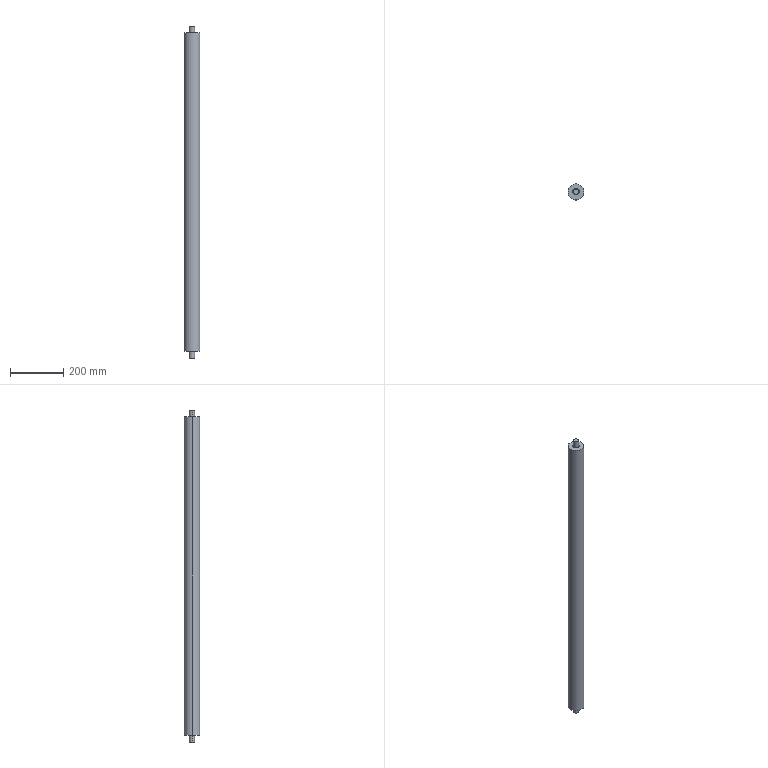Part | SolidWorks | features ICE 2, Extrusion 1, MirrorPattern 1 | 2 solids | 16 faces | box 60 x 60 x 1250 mm | volume 3405863 mm3 | cylinder 10 | plane 6 | commonest cylinder face diameters 20 x4 24 x4 60 x2
STEP:
#1=CARTESIAN_POINT('',(10.,0.,625.));
#2=VERTEX_POINT('',#1);
#3=CARTESIAN_POINT('',(-10.,0.,625.));
#4=VERTEX_POINT('',#3);
#5=CARTESIAN_POINT('',(0.,0.,625.));
#6=DIRECTION('',(0.,0.,1.));
#7=DIRECTION('',(1.,0.,0.));
#8=AXIS2_PLACEMENT_3D('',#5,#6,#7);
#9=CIRCLE('',#8,10.);
#10=EDGE_CURVE('',#2,#4,#9,.T.);
#11=ORIENTED_EDGE('',*,*,#10,.F.);
#12=CARTESIAN_POINT('',(10.,0.,-625.));
#13=VERTEX_POINT('',#12);
#14=CARTESIAN_POINT('',(10.,0.,625.));
#15=DIRECTION('',(0.,0.,-1.));
#16=VECTOR('',#15,1000.);
#17=LINE('',#14,#16);
#18=EDGE_CURVE('',#2,#13,#17,.T.);
#19=ORIENTED_EDGE('',*,*,#18,.T.);
#20=CARTESIAN_POINT('',(-10.,0.,-625.));
#21=VERTEX_POINT('',#20);
#22=CARTESIAN_POINT('',(0.,0.,-625.));
#23=DIRECTION('',(0.,0.,1.));
#24=DIRECTION('',(1.,0.,0.));
#25=AXIS2_PLACEMENT_3D('',#22,#23,#24);
#26=CIRCLE('',#25,10.);
#27=EDGE_CURVE('',#13,#21,#26,.T.);
#28=ORIENTED_EDGE('',*,*,#27,.T.);
#29=CARTESIAN_POINT('',(-10.,0.,625.));
#30=DIRECTION('',(0.,0.,-1.));
#31=VECTOR('',#30,1000.);
#32=LINE('',#29,#31);
#33=EDGE_CURVE('',#4,#21,#32,.T.);
#34=ORIENTED_EDGE('',*,*,#33,.F.);
#35=EDGE_LOOP('',(#11,#19,#28,#34));
#36=FACE_OUTER_BOUND('',#35,.T.);
#37=CARTESIAN_POINT('',(0.,0.,625.));
#38=DIRECTION('',(0.,0.,-1.));
#39=DIRECTION('',(-1.,0.,0.));
#40=AXIS2_PLACEMENT_3D('',#37,#38,#39);
#41=CYLINDRICAL_SURFACE('',#40,10.);
#42=ADVANCED_FACE('',(#36),#41,.T.);
#43=ORIENTED_EDGE('',*,*,#18,.F.);
#44=CARTESIAN_POINT('',(0.,0.,625.));
#45=DIRECTION('',(0.,0.,1.));
#46=DIRECTION('',(1.,0.,0.));
#47=AXIS2_PLACEMENT_3D('',#44,#45,#46);
#48=CIRCLE('',#47,10.);
#49=EDGE_CURVE('',#4,#2,#48,.T.);
#50=ORIENTED_EDGE('',*,*,#49,.F.);
#51=ORIENTED_EDGE('',*,*,#33,.T.);
#52=CARTESIAN_POINT('',(0.,0.,-625.));
#53=DIRECTION('',(0.,0.,1.));
#54=DIRECTION('',(1.,0.,0.));
#55=AXIS2_PLACEMENT_3D('',#52,#53,#54);
#56=CIRCLE('',#55,10.);
#57=EDGE_CURVE('',#21,#13,#56,.T.);
#58=ORIENTED_EDGE('',*,*,#57,.T.);
#59=EDGE_LOOP('',(#43,#50,#51,#58));
#60=FACE_OUTER_BOUND('',#59,.T.);
#61=CARTESIAN_POINT('',(0.,0.,625.));
#62=DIRECTION('',(0.,0.,-1.));
#63=DIRECTION('',(-1.,0.,0.));
#64=AXIS2_PLACEMENT_3D('',#61,#62,#63);
#65=CYLINDRICAL_SURFACE('',#64,10.);
#66=ADVANCED_FACE('',(#60),#65,.T.);
#67=ORIENTED_EDGE('',*,*,#49,.T.);
#68=ORIENTED_EDGE('',*,*,#10,.T.);
#69=EDGE_LOOP('',(#67,#68));
#70=FACE_OUTER_BOUND('',#69,.T.);
#71=CARTESIAN_POINT('',(0.,0.,625.));
#72=DIRECTION('',(0.,0.,1.));
#73=DIRECTION('',(1.,0.,0.));
#74=AXIS2_PLACEMENT_3D('',#71,#72,#73);
#75=PLANE('',#74);
#76=ADVANCED_FACE('',(#70),#75,.T.);
#77=ORIENTED_EDGE('',*,*,#57,.F.);
#78=ORIENTED_EDGE('',*,*,#27,.F.);
#79=EDGE_LOOP('',(#77,#78));
#80=FACE_OUTER_BOUND('',#79,.T.);
#81=CARTESIAN_POINT('',(0.,0.,-625.));
#82=DIRECTION('',(0.,0.,1.));
#83=DIRECTION('',(1.,0.,0.));
#84=AXIS2_PLACEMENT_3D('',#81,#82,#83);
#85=PLANE('',#84);
#86=ADVANCED_FACE('',(#80),#85,.F.);
#87=CLOSED_SHELL('',(#42,#66,#76,#86));
#88=MANIFOLD_SOLID_BREP('',#87);
#89=CARTESIAN_POINT('',(-12.,0.,-590.));
#90=VERTEX_POINT('',#89);
#91=CARTESIAN_POINT('',(12.,0.,-590.));
#92=VERTEX_POINT('',#91);
#93=CARTESIAN_POINT('',(0.,0.,-590.));
#94=DIRECTION('',(0.,0.,1.));
#95=DIRECTION('',(1.,0.,0.));
#96=AXIS2_PLACEMENT_3D('',#93,#94,#95);
#97=CIRCLE('',#96,12.);
#98=EDGE_CURVE('',#90,#92,#97,.T.);
#99=ORIENTED_EDGE('',*,*,#98,.T.);
#100=CARTESIAN_POINT('',(12.,0.,-600.));
#101=VERTEX_POINT('',#100);
#102=CARTESIAN_POINT('',(12.,0.,-590.));
#103=DIRECTION('',(0.,0.,-1.));
#104=VECTOR('',#103,1000.);
#105=LINE('',#102,#104);
#106=EDGE_CURVE('',#92,#101,#105,.T.);
#107=ORIENTED_EDGE('',*,*,#106,.T.);
#108=CARTESIAN_POINT('',(-12.,0.,-600.));
#109=VERTEX_POINT('',#108);
#110=CARTESIAN_POINT('',(0.,0.,-600.));
#111=DIRECTION('',(0.,0.,1.));
#112=DIRECTION('',(1.,0.,0.));
#113=AXIS2_PLACEMENT_3D('',#110,#111,#112);
#114=CIRCLE('',#113,12.);
#115=EDGE_CURVE('',#109,#101,#114,.T.);
#116=ORIENTED_EDGE('',*,*,#115,.F.);
#117=CARTESIAN_POINT('',(-12.,0.,-590.));
#118=DIRECTION('',(0.,0.,-1.));
#119=VECTOR('',#118,1000.);
#120=LINE('',#117,#119);
#121=EDGE_CURVE('',#90,#109,#120,.T.);
#122=ORIENTED_EDGE('',*,*,#121,.F.);
#123=EDGE_LOOP('',(#99,#107,#116,#122));
#124=FACE_OUTER_BOUND('',#123,.T.);
#125=CARTESIAN_POINT('',(0.,0.,-590.));
#126=DIRECTION('',(0.,0.,-1.));
#127=DIRECTION('',(-1.,0.,0.));
#128=AXIS2_PLACEMENT_3D('',#125,#126,#127);
#129=CYLINDRICAL_SURFACE('',#128,12.);
#130=ADVANCED_FACE('',(#124),#129,.F.);
#131=CARTESIAN_POINT('',(-12.,0.,590.));
#132=VERTEX_POINT('',#131);
#133=CARTESIAN_POINT('',(12.,0.,590.));
#134=VERTEX_POINT('',#133);
#135=CARTESIAN_POINT('',(0.,0.,590.));
#136=DIRECTION('',(0.,0.,1.));
#137=DIRECTION('',(1.,0.,0.));
#138=AXIS2_PLACEMENT_3D('',#135,#136,#137);
#139=CIRCLE('',#138,12.);
#140=EDGE_CURVE('',#132,#134,#139,.T.);
#141=ORIENTED_EDGE('',*,*,#140,.F.);
#142=CARTESIAN_POINT('',(-12.,0.,600.));
#143=VERTEX_POINT('',#142);
#144=CARTESIAN_POINT('',(-12.,0.,590.));
#145=DIRECTION('',(0.,0.,1.));
#146=VECTOR('',#145,1000.);
#147=LINE('',#144,#146);
#148=EDGE_CURVE('',#132,#143,#147,.T.);
#149=ORIENTED_EDGE('',*,*,#148,.T.);
#150=CARTESIAN_POINT('',(12.,0.,600.));
#151=VERTEX_POINT('',#150);
#152=CARTESIAN_POINT('',(0.,0.,600.));
#153=DIRECTION('',(0.,0.,1.));
#154=DIRECTION('',(1.,0.,0.));
#155=AXIS2_PLACEMENT_3D('',#152,#153,#154);
#156=CIRCLE('',#155,12.);
#157=EDGE_CURVE('',#143,#151,#156,.T.);
#158=ORIENTED_EDGE('',*,*,#157,.T.);
#159=CARTESIAN_POINT('',(12.,0.,590.));
#160=DIRECTION('',(0.,0.,1.));
#161=VECTOR('',#160,1000.);
#162=LINE('',#159,#161);
#163=EDGE_CURVE('',#134,#151,#162,.T.);
#164=ORIENTED_EDGE('',*,*,#163,.F.);
#165=EDGE_LOOP('',(#141,#149,#158,#164));
#166=FACE_OUTER_BOUND('',#165,.T.);
#167=CARTESIAN_POINT('',(0.,0.,590.));
#168=DIRECTION('',(0.,0.,1.));
#169=DIRECTION('',(1.,0.,0.));
#170=AXIS2_PLACEMENT_3D('',#167,#168,#169);
#171=CYLINDRICAL_SURFACE('',#170,12.);
#172=ADVANCED_FACE('',(#166),#171,.F.);
#173=CARTESIAN_POINT('',(30.,0.,600.));
#174=VERTEX_POINT('',#173);
#175=CARTESIAN_POINT('',(-30.,0.,600.));
#176=VERTEX_POINT('',#175);
#177=CARTESIAN_POINT('',(0.,0.,600.));
#178=DIRECTION('',(0.,0.,1.));
#179=DIRECTION('',(1.,0.,0.));
#180=AXIS2_PLACEMENT_3D('',#177,#178,#179);
#181=CIRCLE('',#180,30.);
#182=EDGE_CURVE('',#174,#176,#181,.T.);
#183=ORIENTED_EDGE('',*,*,#182,.F.);
#184=CARTESIAN_POINT('',(30.,0.,-600.));
#185=VERTEX_POINT('',#184);
#186=CARTESIAN_POINT('',(30.,0.,600.));
#187=DIRECTION('',(0.,0.,-1.));
#188=VECTOR('',#187,1000.);
#189=LINE('',#186,#188);
#190=EDGE_CURVE('',#174,#185,#189,.T.);
#191=ORIENTED_EDGE('',*,*,#190,.T.);
#192=CARTESIAN_POINT('',(-30.,0.,-600.));
#193=VERTEX_POINT('',#192);
#194=CARTESIAN_POINT('',(0.,0.,-600.));
#195=DIRECTION('',(0.,0.,1.));
#196=DIRECTION('',(1.,0.,0.));
#197=AXIS2_PLACEMENT_3D('',#194,#195,#196);
#198=CIRCLE('',#197,30.);
#199=EDGE_CURVE('',#185,#193,#198,.T.);
#200=ORIENTED_EDGE('',*,*,#199,.T.);
#201=CARTESIAN_POINT('',(-30.,0.,600.));
#202=DIRECTION('',(0.,0.,-1.));
#203=VECTOR('',#202,1000.);
#204=LINE('',#201,#203);
#205=EDGE_CURVE('',#176,#193,#204,.T.);
#206=ORIENTED_EDGE('',*,*,#205,.F.);
#207=EDGE_LOOP('',(#183,#191,#200,#206));
#208=FACE_OUTER_BOUND('',#207,.T.);
#209=CARTESIAN_POINT('',(0.,0.,600.));
#210=DIRECTION('',(0.,0.,-1.));
#211=DIRECTION('',(-1.,0.,0.));
#212=AXIS2_PLACEMENT_3D('',#209,#210,#211);
#213=CYLINDRICAL_SURFACE('',#212,30.);
#214=ADVANCED_FACE('',(#208),#213,.T.);
#215=CARTESIAN_POINT('',(-10.,0.,590.));
#216=VERTEX_POINT('',#215);
#217=CARTESIAN_POINT('',(10.,0.,590.));
#218=VERTEX_POINT('',#217);
#219=CARTESIAN_POINT('',(0.,0.,590.));
#220=DIRECTION('',(0.,0.,1.));
#221=DIRECTION('',(1.,0.,0.));
#222=AXIS2_PLACEMENT_3D('',#219,#220,#221);
#223=CIRCLE('',#222,10.);
#224=EDGE_CURVE('',#216,#218,#223,.T.);
#225=ORIENTED_EDGE('',*,*,#224,.T.);
#226=CARTESIAN_POINT('',(10.,0.,-590.));
#227=VERTEX_POINT('',#226);
#228=CARTESIAN_POINT('',(10.,0.,600.));
#229=DIRECTION('',(0.,0.,-1.));
#230=VECTOR('',#229,1000.);
#231=LINE('',#228,#230);
#232=EDGE_CURVE('',#218,#227,#231,.T.);
#233=ORIENTED_EDGE('',*,*,#232,.T.);
#234=CARTESIAN_POINT('',(-10.,0.,-590.));
#235=VERTEX_POINT('',#234);
#236=CARTESIAN_POINT('',(0.,0.,-590.));
#237=DIRECTION('',(0.,0.,-1.));
#238=DIRECTION('',(-1.,0.,0.));
#239=AXIS2_PLACEMENT_3D('',#236,#237,#238);
#240=CIRCLE('',#239,10.);
#241=EDGE_CURVE('',#227,#235,#240,.T.);
#242=ORIENTED_EDGE('',*,*,#241,.T.);
#243=CARTESIAN_POINT('',(-10.,0.,600.));
#244=DIRECTION('',(0.,0.,-1.));
#245=VECTOR('',#244,1000.);
#246=LINE('',#243,#245);
#247=EDGE_CURVE('',#216,#235,#246,.T.);
#248=ORIENTED_EDGE('',*,*,#247,.F.);
#249=EDGE_LOOP('',(#225,#233,#242,#248));
#250=FACE_OUTER_BOUND('',#249,.T.);
#251=CARTESIAN_POINT('',(0.,0.,600.));
#252=DIRECTION('',(0.,0.,-1.));
#253=DIRECTION('',(-1.,0.,0.));
#254=AXIS2_PLACEMENT_3D('',#251,#252,#253);
#255=CYLINDRICAL_SURFACE('',#254,10.);
#256=ADVANCED_FACE('',(#250),#255,.F.);
#257=ORIENTED_EDGE('',*,*,#232,.F.);
#258=CARTESIAN_POINT('',(0.,0.,590.));
#259=DIRECTION('',(0.,0.,1.));
#260=DIRECTION('',(1.,0.,0.));
#261=AXIS2_PLACEMENT_3D('',#258,#259,#260);
#262=CIRCLE('',#261,10.);
#263=EDGE_CURVE('',#218,#216,#262,.T.);
#264=ORIENTED_EDGE('',*,*,#263,.T.);
#265=ORIENTED_EDGE('',*,*,#247,.T.);
#266=CARTESIAN_POINT('',(0.,0.,-590.));
#267=DIRECTION('',(0.,0.,-1.));
#268=DIRECTION('',(-1.,0.,0.));
#269=AXIS2_PLACEMENT_3D('',#266,#267,#268);
#270=CIRCLE('',#269,10.);
#271=EDGE_CURVE('',#235,#227,#270,.T.);
#272=ORIENTED_EDGE('',*,*,#271,.T.);
#273=EDGE_LOOP('',(#257,#264,#265,#272));
#274=FACE_OUTER_BOUND('',#273,.T.);
#275=CARTESIAN_POINT('',(0.,0.,600.));
#276=DIRECTION('',(0.,0.,-1.));
#277=DIRECTION('',(-1.,0.,0.));
#278=AXIS2_PLACEMENT_3D('',#275,#276,#277);
#279=CYLINDRICAL_SURFACE('',#278,10.);
#280=ADVANCED_FACE('',(#274),#279,.F.);
#281=CARTESIAN_POINT('',(0.,0.,600.));
#282=DIRECTION('',(0.,0.,1.));
#283=DIRECTION('',(1.,0.,0.));
#284=AXIS2_PLACEMENT_3D('',#281,#282,#283);
#285=CIRCLE('',#284,12.);
#286=EDGE_CURVE('',#151,#143,#285,.T.);
#287=ORIENTED_EDGE('',*,*,#286,.F.);
#288=ORIENTED_EDGE('',*,*,#157,.F.);
#289=EDGE_LOOP('',(#287,#288));
#290=FACE_BOUND('',#289,.T.);
#291=CARTESIAN_POINT('',(0.,0.,600.));
#292=DIRECTION('',(0.,0.,1.));
#293=DIRECTION('',(1.,0.,0.));
#294=AXIS2_PLACEMENT_3D('',#291,#292,#293);
#295=CIRCLE('',#294,30.);
#296=EDGE_CURVE('',#176,#174,#295,.T.);
#297=ORIENTED_EDGE('',*,*,#296,.T.);
#298=ORIENTED_EDGE('',*,*,#182,.T.);
#299=EDGE_LOOP('',(#297,#298));
#300=FACE_OUTER_BOUND('',#299,.T.);
#301=CARTESIAN_POINT('',(0.,0.,600.));
#302=DIRECTION('',(0.,0.,1.));
#303=DIRECTION('',(1.,0.,0.));
#304=AXIS2_PLACEMENT_3D('',#301,#302,#303);
#305=PLANE('',#304);
#306=ADVANCED_FACE('',(#290,#300),#305,.T.);
#307=ORIENTED_EDGE('',*,*,#115,.T.);
#308=CARTESIAN_POINT('',(0.,0.,-600.));
#309=DIRECTION('',(0.,0.,1.));
#310=DIRECTION('',(1.,0.,0.));
#311=AXIS2_PLACEMENT_3D('',#308,#309,#310);
#312=CIRCLE('',#311,12.);
#313=EDGE_CURVE('',#101,#109,#312,.T.);
#314=ORIENTED_EDGE('',*,*,#313,.T.);
#315=EDGE_LOOP('',(#307,#314));
#316=FACE_BOUND('',#315,.T.);
#317=CARTESIAN_POINT('',(0.,0.,-600.));
#318=DIRECTION('',(0.,0.,1.));
#319=DIRECTION('',(1.,0.,0.));
#320=AXIS2_PLACEMENT_3D('',#317,#318,#319);
#321=CIRCLE('',#320,30.);
#322=EDGE_CURVE('',#193,#185,#321,.T.);
#323=ORIENTED_EDGE('',*,*,#322,.F.);
#324=ORIENTED_EDGE('',*,*,#199,.F.);
#325=EDGE_LOOP('',(#323,#324));
#326=FACE_OUTER_BOUND('',#325,.T.);
#327=CARTESIAN_POINT('',(0.,0.,-600.));
#328=DIRECTION('',(0.,0.,1.));
#329=DIRECTION('',(1.,0.,0.));
#330=AXIS2_PLACEMENT_3D('',#327,#328,#329);
#331=PLANE('',#330);
#332=ADVANCED_FACE('',(#316,#326),#331,.F.);
#333=ORIENTED_EDGE('',*,*,#190,.F.);
#334=ORIENTED_EDGE('',*,*,#296,.F.);
#335=ORIENTED_EDGE('',*,*,#205,.T.);
#336=ORIENTED_EDGE('',*,*,#322,.T.);
#337=EDGE_LOOP('',(#333,#334,#335,#336));
#338=FACE_OUTER_BOUND('',#337,.T.);
#339=CARTESIAN_POINT('',(0.,0.,600.));
#340=DIRECTION('',(0.,0.,-1.));
#341=DIRECTION('',(-1.,0.,0.));
#342=AXIS2_PLACEMENT_3D('',#339,#340,#341);
#343=CYLINDRICAL_SURFACE('',#342,30.);
#344=ADVANCED_FACE('',(#338),#343,.T.);
#345=ORIENTED_EDGE('',*,*,#148,.F.);
#346=CARTESIAN_POINT('',(0.,0.,590.));
#347=DIRECTION('',(0.,0.,1.));
#348=DIRECTION('',(1.,0.,0.));
#349=AXIS2_PLACEMENT_3D('',#346,#347,#348);
#350=CIRCLE('',#349,12.);
#351=EDGE_CURVE('',#134,#132,#350,.T.);
#352=ORIENTED_EDGE('',*,*,#351,.F.);
#353=ORIENTED_EDGE('',*,*,#163,.T.);
#354=ORIENTED_EDGE('',*,*,#286,.T.);
#355=EDGE_LOOP('',(#345,#352,#353,#354));
#356=FACE_OUTER_BOUND('',#355,.T.);
#357=CARTESIAN_POINT('',(0.,0.,590.));
#358=DIRECTION('',(0.,0.,1.));
#359=DIRECTION('',(1.,0.,0.));
#360=AXIS2_PLACEMENT_3D('',#357,#358,#359);
#361=CYLINDRICAL_SURFACE('',#360,12.);
#362=ADVANCED_FACE('',(#356),#361,.F.);
#363=ORIENTED_EDGE('',*,*,#224,.F.);
#364=ORIENTED_EDGE('',*,*,#263,.F.);
#365=EDGE_LOOP('',(#363,#364));
#366=FACE_BOUND('',#365,.T.);
#367=ORIENTED_EDGE('',*,*,#351,.T.);
#368=ORIENTED_EDGE('',*,*,#140,.T.);
#369=EDGE_LOOP('',(#367,#368));
#370=FACE_OUTER_BOUND('',#369,.T.);
#371=CARTESIAN_POINT('',(0.,0.,590.));
#372=DIRECTION('',(0.,0.,1.));
#373=DIRECTION('',(1.,0.,0.));
#374=AXIS2_PLACEMENT_3D('',#371,#372,#373);
#375=PLANE('',#374);
#376=ADVANCED_FACE('',(#366,#370),#375,.T.);
#377=ORIENTED_EDGE('',*,*,#271,.F.);
#378=ORIENTED_EDGE('',*,*,#241,.F.);
#379=EDGE_LOOP('',(#377,#378));
#380=FACE_BOUND('',#379,.T.);
#381=ORIENTED_EDGE('',*,*,#98,.F.);
#382=CARTESIAN_POINT('',(0.,0.,-590.));
#383=DIRECTION('',(0.,0.,1.));
#384=DIRECTION('',(1.,0.,0.));
#385=AXIS2_PLACEMENT_3D('',#382,#383,#384);
#386=CIRCLE('',#385,12.);
#387=EDGE_CURVE('',#92,#90,#386,.T.);
#388=ORIENTED_EDGE('',*,*,#387,.F.);
#389=EDGE_LOOP('',(#381,#388));
#390=FACE_OUTER_BOUND('',#389,.T.);
#391=CARTESIAN_POINT('',(0.,0.,-590.));
#392=DIRECTION('',(0.,0.,-1.));
#393=DIRECTION('',(1.,0.,0.));
#394=AXIS2_PLACEMENT_3D('',#391,#392,#393);
#395=PLANE('',#394);
#396=ADVANCED_FACE('',(#380,#390),#395,.T.);
#397=ORIENTED_EDGE('',*,*,#106,.F.);
#398=ORIENTED_EDGE('',*,*,#387,.T.);
#399=ORIENTED_EDGE('',*,*,#121,.T.);
#400=ORIENTED_EDGE('',*,*,#313,.F.);
#401=EDGE_LOOP('',(#397,#398,#399,#400));
#402=FACE_OUTER_BOUND('',#401,.T.);
#403=CARTESIAN_POINT('',(0.,0.,-590.));
#404=DIRECTION('',(0.,0.,-1.));
#405=DIRECTION('',(-1.,0.,0.));
#406=AXIS2_PLACEMENT_3D('',#403,#404,#405);
#407=CYLINDRICAL_SURFACE('',#406,12.);
#408=ADVANCED_FACE('',(#402),#407,.F.);
#409=CLOSED_SHELL('',(#130,#172,#214,#256,#280,#306,#332,#344,#362,#376,#396,#408));
#410=MANIFOLD_SOLID_BREP('',#409);
#411=CARTESIAN_POINT('',(0.,0.,0.));
#412=DIRECTION('',(0.,0.,1.));
#413=DIRECTION('',(1.,0.,0.));
#414=AXIS2_PLACEMENT_3D('',#411,#412,#413);
#415=(LENGTH_UNIT()NAMED_UNIT(*)SI_UNIT(.MILLI.,.METRE.));
#416=UNCERTAINTY_MEASURE_WITH_UNIT(LENGTH_MEASURE(0.00001),#415,'','');
#417=(NAMED_UNIT(*)PLANE_ANGLE_UNIT()SI_UNIT($,.RADIAN.));
#418=(NAMED_UNIT(*)SI_UNIT($,.STERADIAN.)SOLID_ANGLE_UNIT());
#419=(GEOMETRIC_REPRESENTATION_CONTEXT(3)GLOBAL_UNCERTAINTY_ASSIGNED_CONTEXT((#416))GLOBAL_UNIT_ASSIGNED_CONTEXT((#415,#417,#418))REPRESENTATION_CONTEXT('',''));
#420=ADVANCED_BREP_SHAPE_REPRESENTATION('',(#88,#410,#414),#419);